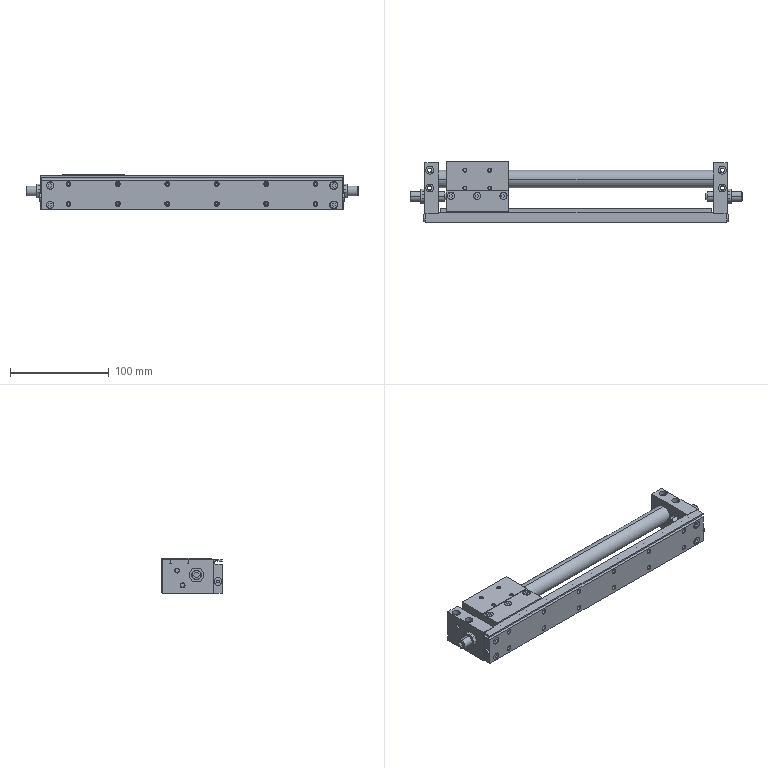Part | SolidWorks | features BaseBody 4, MoveFace 1 | 4 solids | 403 faces | box 336 x 61 x 36 mm | volume 312285 mm3 | plane 182 | cylinder 137 | cone 84 | commonest cylinder face diameters 4.134 x36 3.242 x16 7 x14 7.5 x14 14.8 x12 4.5 x8